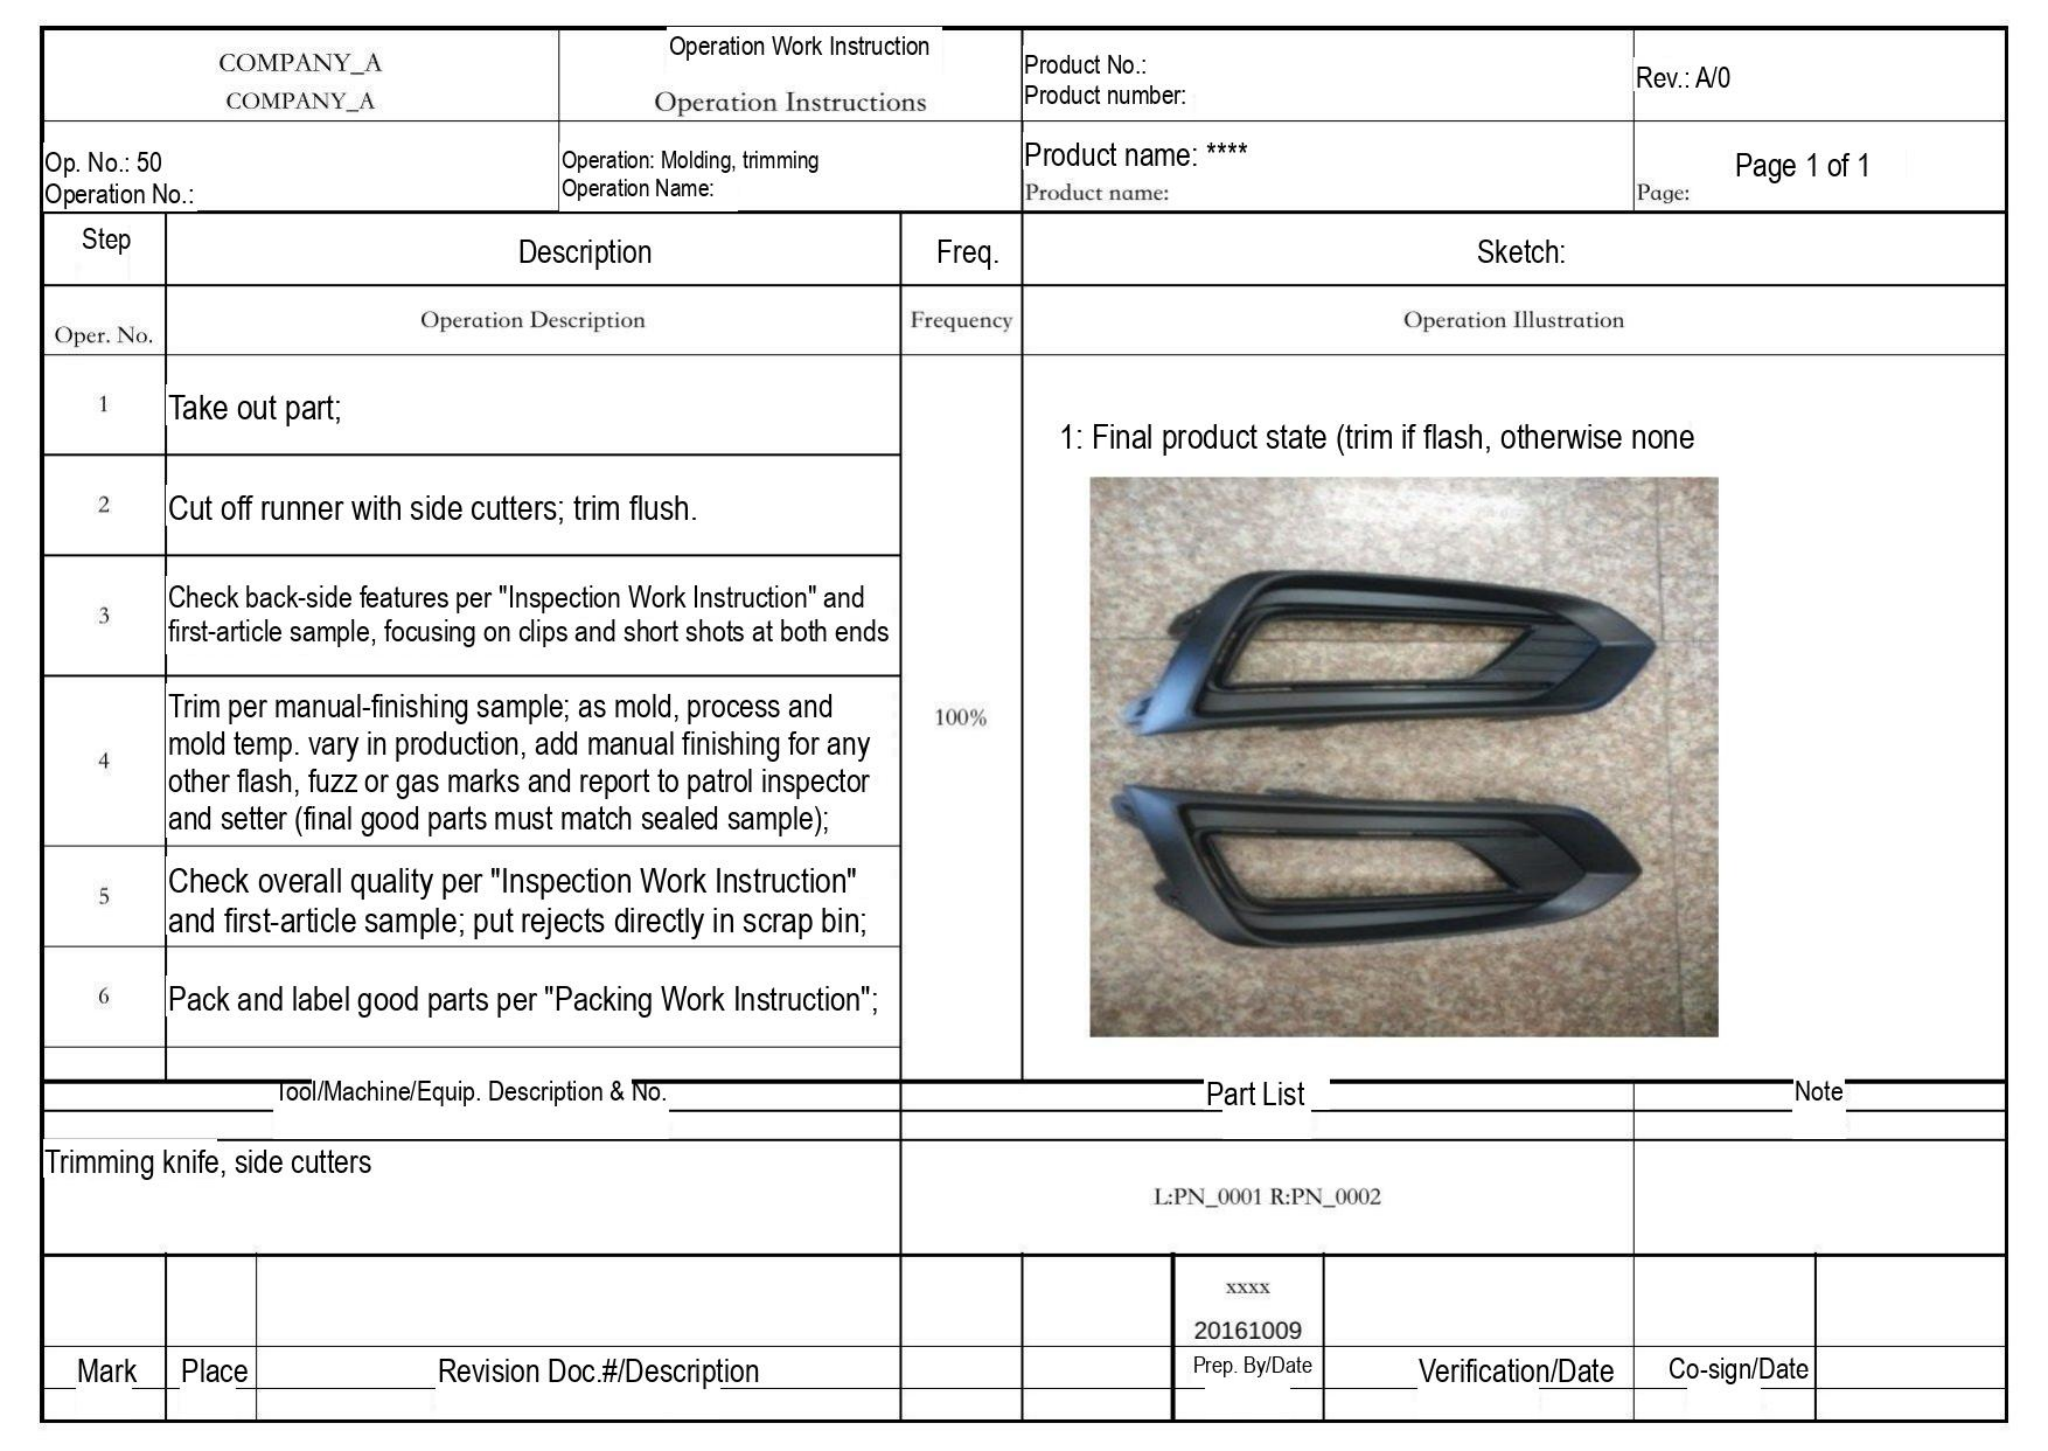| COMPANY_A<br>COMPANY_A | Operation Work Instruction<br>Operation Instructions | Product No.:<br>Product number: | Rev.: A/0 |
|---|---|---|---|
| Op. No.: 50<br>Operation No.: | Operation: Molding, trimming<br>Operation Name: | Product name: ****<br>Product name: | Page 1 of 1<br>Page: |

| Step<br>Oper. No. | Description<br>Operation Description | Freq.<br>Frequency | Sketch:<br>Operation Illustration |
|---|---|---|---|
| 1 | Take out part; | 100% | 1: Final product state (trim if flash, otherwise none |
| 2 | Cut off runner with side cutters; trim flush. | | |
| 3 | Check back-side features per "Inspection Work Instruction" and first-article sample, focusing on clips and short shots at both ends | | |
| 4 | Trim per manual-finishing sample; as mold, process and mold temp. vary in production, add manual finishing for any other flash, fuzz or gas marks and report to patrol inspector and setter (final good parts must match sealed sample); | | |
| 5 | Check overall quality per "Inspection Work Instruction" and first-article sample; put rejects directly in scrap bin; | | |
| 6 | Pack and label good parts per "Packing Work Instruction"; | | |

| Tool/Machine/Equip. Description & No. | Part List | Note |
|---|---|---|
| Trimming knife, side cutters | L:PN_0001 R:PN_0002 | |

| Mark | Place | Revision Doc.#/Description | | | xxxx<br>20161009<br>Prep. By/Date | Verification/Date | Co-sign/Date | |
|---|---|---|---|---|---|---|---|---|